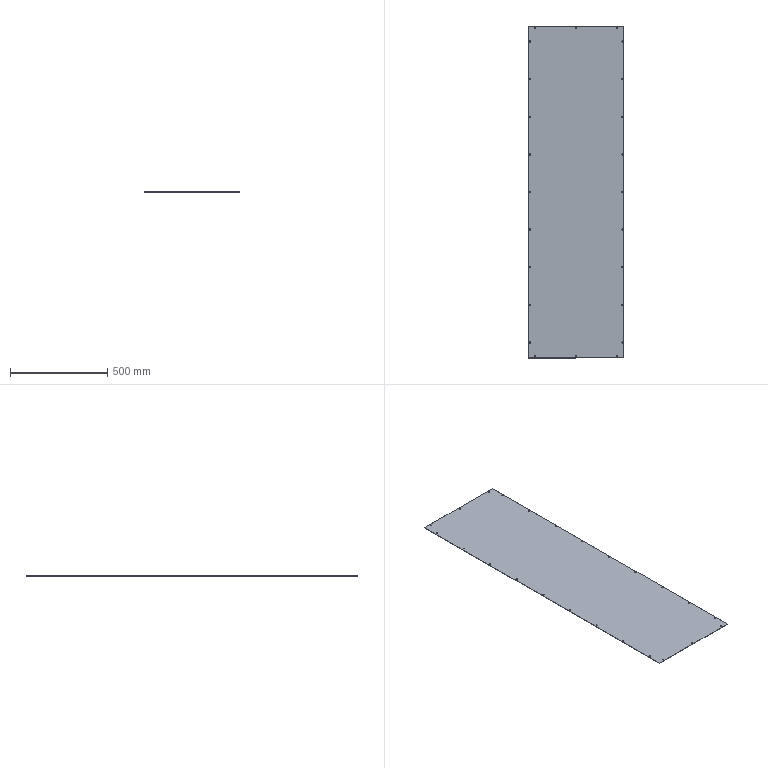Part | SolidWorks | 1 solid | 54 faces | box 492 x 1703 x 2 mm | volume 1674159 mm3 | cylinder 48 | plane 6 | commonest cylinder face diameters 6.5 x48